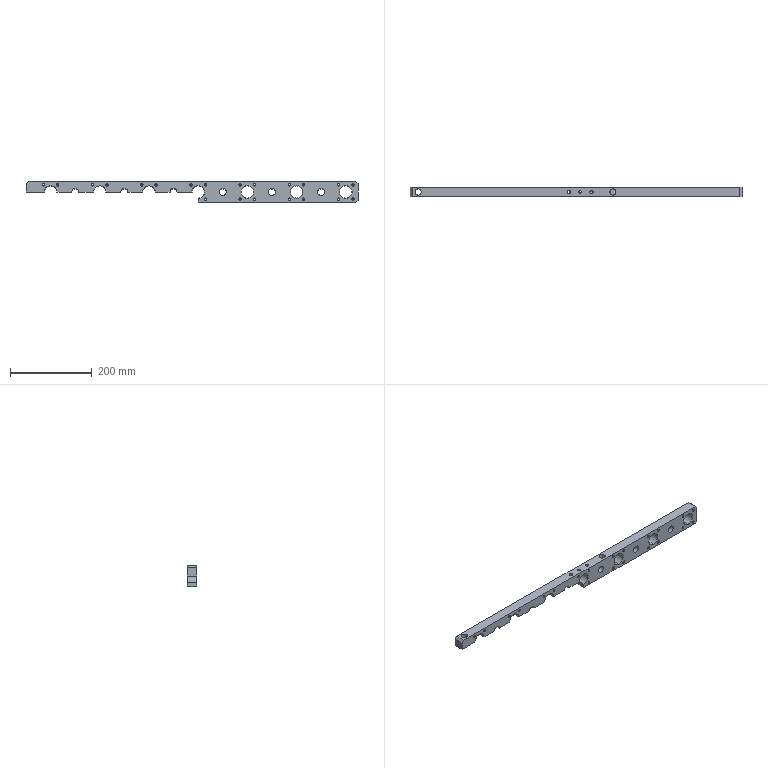Part | STEP file | Cuon T phu H01_1 | 1 solid | 223 faces | box 810 x 24 x 50 mm | volume 584750 mm3 | cone 112 | cylinder 75 | plane 36 | commonest cylinder face diameters 5 x42 30 x14 17 x9 8.5 x4 15 x4 6 x2